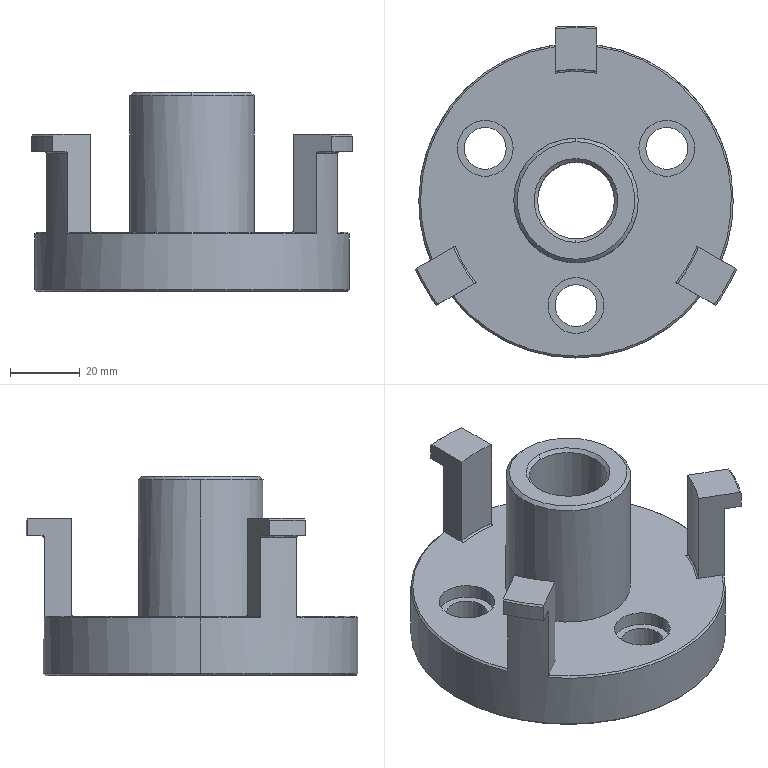Part | STEP file | Rotor locating claw-PN_0001 | 1 solid | 88 faces | box 91.977 x 95 x 57 mm | volume 127328 mm3 | cylinder 38 | cone 23 | plane 21 | spline 6 | commonest cylinder face diameters 3.3 x8 4 x6 12 x6 16 x6 75 x3 100 x3